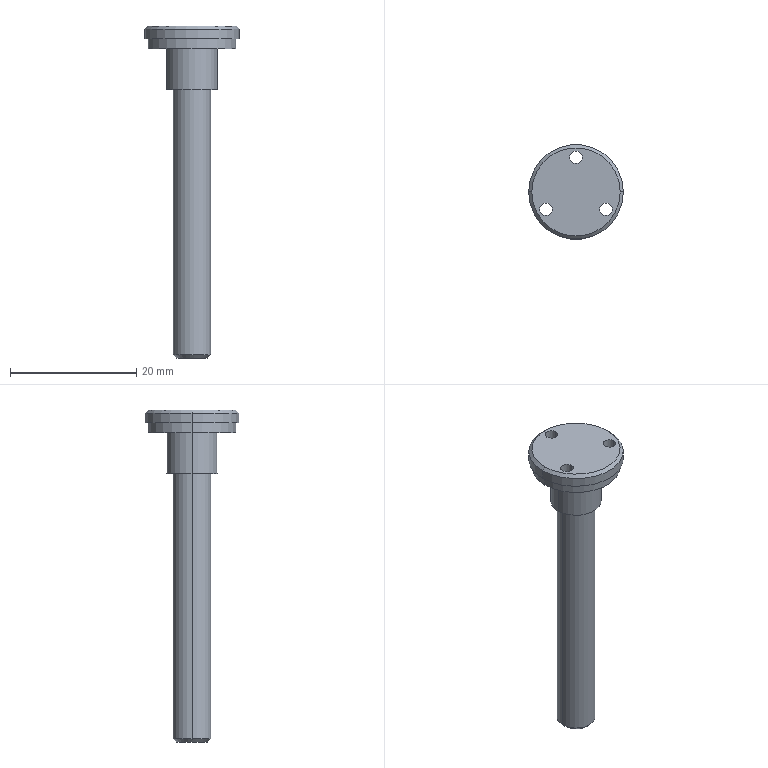Part | NX | features BREP 1 | 1 solid | 26 faces | box 15 x 15 x 52.6 mm | volume 2030 mm3 | cylinder 16 | plane 6 | cone 4 | commonest cylinder face diameters 2 x6 3.1 x2 6 x2 8 x2 13.9 x2 15 x2
STEP:
#1=CARTESIAN_POINT('',(-165.024,187.29,-49.6));
#2=VERTEX_POINT('',#1);
#3=CARTESIAN_POINT('',(-160.024,187.29,-49.6));
#4=VERTEX_POINT('',#3);
#5=CARTESIAN_POINT('',(-162.524,187.29,-49.6));
#6=DIRECTION('',(0.,0.,-1.));
#7=DIRECTION('',(1.,0.,0.));
#8=AXIS2_PLACEMENT_3D('',#5,#6,#7);
#9=CIRCLE('',#8,2.5);
#10=EDGE_CURVE('',#2,#4,#9,.T.);
#11=ORIENTED_EDGE('',*,*,#10,.F.);
#12=CARTESIAN_POINT('',(-165.524,187.29,-49.1));
#13=VERTEX_POINT('',#12);
#14=CARTESIAN_POINT('',(-165.024,187.29,-49.6));
#15=DIRECTION('',(-0.7071,0.,0.7071));
#16=VECTOR('',#15,1000.);
#17=LINE('',#14,#16);
#18=EDGE_CURVE('',#2,#13,#17,.T.);
#19=ORIENTED_EDGE('',*,*,#18,.T.);
#20=CARTESIAN_POINT('',(-159.524,187.29,-49.1));
#21=VERTEX_POINT('',#20);
#22=CARTESIAN_POINT('',(-162.524,187.29,-49.1));
#23=DIRECTION('',(0.,0.,1.));
#24=DIRECTION('',(1.,0.,0.));
#25=AXIS2_PLACEMENT_3D('',#22,#23,#24);
#26=CIRCLE('',#25,3.);
#27=EDGE_CURVE('',#21,#13,#26,.T.);
#28=ORIENTED_EDGE('',*,*,#27,.F.);
#29=CARTESIAN_POINT('',(-160.024,187.29,-49.6));
#30=DIRECTION('',(0.7071,0.,0.7071));
#31=VECTOR('',#30,1000.);
#32=LINE('',#29,#31);
#33=EDGE_CURVE('',#4,#21,#32,.T.);
#34=ORIENTED_EDGE('',*,*,#33,.F.);
#35=EDGE_LOOP('',(#11,#19,#28,#34));
#36=FACE_BOUND('',#35,.T.);
#37=CARTESIAN_POINT('',(-162.524,187.29,-49.6));
#38=DIRECTION('',(0.,0.,1.));
#39=DIRECTION('',(-1.,0.,0.));
#40=AXIS2_PLACEMENT_3D('',#37,#38,#39);
#41=CONICAL_SURFACE('',#40,2.5,0.7854);
#42=ADVANCED_FACE('',(#36),#41,.T.);
#43=CARTESIAN_POINT('',(-155.524,187.29,3.));
#44=VERTEX_POINT('',#43);
#45=CARTESIAN_POINT('',(-169.524,187.29,3.));
#46=VERTEX_POINT('',#45);
#47=CARTESIAN_POINT('',(-162.524,187.29,3.));
#48=DIRECTION('',(0.,0.,1.));
#49=DIRECTION('',(1.,0.,0.));
#50=AXIS2_PLACEMENT_3D('',#47,#48,#49);
#51=CIRCLE('',#50,7.);
#52=EDGE_CURVE('',#44,#46,#51,.T.);
#53=ORIENTED_EDGE('',*,*,#52,.F.);
#54=CARTESIAN_POINT('',(-155.024,187.29,2.5));
#55=VERTEX_POINT('',#54);
#56=CARTESIAN_POINT('',(-155.524,187.29,3.));
#57=DIRECTION('',(0.7071,0.,-0.7071));
#58=VECTOR('',#57,1000.);
#59=LINE('',#56,#58);
#60=EDGE_CURVE('',#55,#44,#59,.F.);
#61=ORIENTED_EDGE('',*,*,#60,.F.);
#62=CARTESIAN_POINT('',(-170.024,187.29,2.5));
#63=VERTEX_POINT('',#62);
#64=CARTESIAN_POINT('',(-162.524,187.29,2.5));
#65=DIRECTION('',(0.,0.,-1.));
#66=DIRECTION('',(1.,0.,0.));
#67=AXIS2_PLACEMENT_3D('',#64,#65,#66);
#68=CIRCLE('',#67,7.5);
#69=EDGE_CURVE('',#63,#55,#68,.T.);
#70=ORIENTED_EDGE('',*,*,#69,.F.);
#71=CARTESIAN_POINT('',(-169.524,187.29,3.));
#72=DIRECTION('',(-0.7071,0.,-0.7071));
#73=VECTOR('',#72,1000.);
#74=LINE('',#71,#73);
#75=EDGE_CURVE('',#63,#46,#74,.F.);
#76=ORIENTED_EDGE('',*,*,#75,.T.);
#77=EDGE_LOOP('',(#53,#61,#70,#76));
#78=FACE_BOUND('',#77,.T.);
#79=CARTESIAN_POINT('',(-162.524,187.29,3.));
#80=DIRECTION('',(0.,0.,-1.));
#81=DIRECTION('',(1.,0.,0.));
#82=AXIS2_PLACEMENT_3D('',#79,#80,#81);
#83=CONICAL_SURFACE('',#82,7.,0.7854);
#84=ADVANCED_FACE('',(#78),#83,.T.);
#85=CARTESIAN_POINT('',(-163.524,192.79,3.));
#86=VERTEX_POINT('',#85);
#87=CARTESIAN_POINT('',(-161.524,192.79,3.));
#88=VERTEX_POINT('',#87);
#89=CARTESIAN_POINT('',(-162.524,192.79,3.));
#90=DIRECTION('',(0.,0.,1.));
#91=DIRECTION('',(1.,0.,0.));
#92=AXIS2_PLACEMENT_3D('',#89,#90,#91);
#93=CIRCLE('',#92,1.);
#94=EDGE_CURVE('',#86,#88,#93,.T.);
#95=ORIENTED_EDGE('',*,*,#94,.T.);
#96=CARTESIAN_POINT('',(-161.524,192.79,-0.6));
#97=VERTEX_POINT('',#96);
#98=CARTESIAN_POINT('',(-161.524,192.79,9.4));
#99=DIRECTION('',(0.,0.,-1.));
#100=VECTOR('',#99,1000.);
#101=LINE('',#98,#100);
#102=EDGE_CURVE('',#97,#88,#101,.F.);
#103=ORIENTED_EDGE('',*,*,#102,.F.);
#104=CARTESIAN_POINT('',(-163.524,192.79,-0.6));
#105=VERTEX_POINT('',#104);
#106=CARTESIAN_POINT('',(-162.524,192.79,-0.6));
#107=DIRECTION('',(0.,0.,-1.));
#108=DIRECTION('',(-1.,0.,0.));
#109=AXIS2_PLACEMENT_3D('',#106,#107,#108);
#110=CIRCLE('',#109,1.);
#111=EDGE_CURVE('',#97,#105,#110,.T.);
#112=ORIENTED_EDGE('',*,*,#111,.T.);
#113=CARTESIAN_POINT('',(-163.524,192.79,9.4));
#114=DIRECTION('',(0.,0.,-1.));
#115=VECTOR('',#114,1000.);
#116=LINE('',#113,#115);
#117=EDGE_CURVE('',#105,#86,#116,.F.);
#118=ORIENTED_EDGE('',*,*,#117,.T.);
#119=EDGE_LOOP('',(#95,#103,#112,#118));
#120=FACE_BOUND('',#119,.T.);
#121=CARTESIAN_POINT('',(-162.524,192.79,9.4));
#122=DIRECTION('',(0.,0.,-1.));
#123=DIRECTION('',(1.,0.,0.));
#124=AXIS2_PLACEMENT_3D('',#121,#122,#123);
#125=CYLINDRICAL_SURFACE('',#124,1.);
#126=ADVANCED_FACE('',(#120),#125,.F.);
#127=CARTESIAN_POINT('',(-168.288,184.54,3.));
#128=VERTEX_POINT('',#127);
#129=CARTESIAN_POINT('',(-166.288,184.54,3.));
#130=VERTEX_POINT('',#129);
#131=CARTESIAN_POINT('',(-167.288,184.54,3.));
#132=DIRECTION('',(0.,0.,1.));
#133=DIRECTION('',(1.,0.,0.));
#134=AXIS2_PLACEMENT_3D('',#131,#132,#133);
#135=CIRCLE('',#134,1.);
#136=EDGE_CURVE('',#128,#130,#135,.T.);
#137=ORIENTED_EDGE('',*,*,#136,.T.);
#138=CARTESIAN_POINT('',(-166.288,184.54,-0.6));
#139=VERTEX_POINT('',#138);
#140=CARTESIAN_POINT('',(-166.288,184.54,9.4));
#141=DIRECTION('',(0.,0.,-1.));
#142=VECTOR('',#141,1000.);
#143=LINE('',#140,#142);
#144=EDGE_CURVE('',#139,#130,#143,.F.);
#145=ORIENTED_EDGE('',*,*,#144,.F.);
#146=CARTESIAN_POINT('',(-168.288,184.54,-0.6));
#147=VERTEX_POINT('',#146);
#148=CARTESIAN_POINT('',(-167.288,184.54,-0.6));
#149=DIRECTION('',(0.,0.,-1.));
#150=DIRECTION('',(-1.,0.,0.));
#151=AXIS2_PLACEMENT_3D('',#148,#149,#150);
#152=CIRCLE('',#151,1.);
#153=EDGE_CURVE('',#139,#147,#152,.T.);
#154=ORIENTED_EDGE('',*,*,#153,.T.);
#155=CARTESIAN_POINT('',(-168.288,184.54,9.4));
#156=DIRECTION('',(0.,0.,-1.));
#157=VECTOR('',#156,1000.);
#158=LINE('',#155,#157);
#159=EDGE_CURVE('',#147,#128,#158,.F.);
#160=ORIENTED_EDGE('',*,*,#159,.T.);
#161=EDGE_LOOP('',(#137,#145,#154,#160));
#162=FACE_BOUND('',#161,.T.);
#163=CARTESIAN_POINT('',(-167.288,184.54,9.4));
#164=DIRECTION('',(0.,0.,-1.));
#165=DIRECTION('',(1.,0.,0.));
#166=AXIS2_PLACEMENT_3D('',#163,#164,#165);
#167=CYLINDRICAL_SURFACE('',#166,1.);
#168=ADVANCED_FACE('',(#162),#167,.F.);
#169=CARTESIAN_POINT('',(-158.761,184.54,3.));
#170=VERTEX_POINT('',#169);
#171=CARTESIAN_POINT('',(-156.761,184.54,3.));
#172=VERTEX_POINT('',#171);
#173=CARTESIAN_POINT('',(-157.761,184.54,3.));
#174=DIRECTION('',(0.,0.,1.));
#175=DIRECTION('',(1.,0.,0.));
#176=AXIS2_PLACEMENT_3D('',#173,#174,#175);
#177=CIRCLE('',#176,1.);
#178=EDGE_CURVE('',#170,#172,#177,.T.);
#179=ORIENTED_EDGE('',*,*,#178,.T.);
#180=CARTESIAN_POINT('',(-156.761,184.54,-0.6));
#181=VERTEX_POINT('',#180);
#182=CARTESIAN_POINT('',(-156.761,184.54,9.4));
#183=DIRECTION('',(0.,0.,-1.));
#184=VECTOR('',#183,1000.);
#185=LINE('',#182,#184);
#186=EDGE_CURVE('',#181,#172,#185,.F.);
#187=ORIENTED_EDGE('',*,*,#186,.F.);
#188=CARTESIAN_POINT('',(-158.761,184.54,-0.6));
#189=VERTEX_POINT('',#188);
#190=CARTESIAN_POINT('',(-157.761,184.54,-0.6));
#191=DIRECTION('',(0.,0.,-1.));
#192=DIRECTION('',(-1.,0.,0.));
#193=AXIS2_PLACEMENT_3D('',#190,#191,#192);
#194=CIRCLE('',#193,1.);
#195=EDGE_CURVE('',#181,#189,#194,.T.);
#196=ORIENTED_EDGE('',*,*,#195,.T.);
#197=CARTESIAN_POINT('',(-158.761,184.54,9.4));
#198=DIRECTION('',(0.,0.,-1.));
#199=VECTOR('',#198,1000.);
#200=LINE('',#197,#199);
#201=EDGE_CURVE('',#189,#170,#200,.F.);
#202=ORIENTED_EDGE('',*,*,#201,.T.);
#203=EDGE_LOOP('',(#179,#187,#196,#202));
#204=FACE_BOUND('',#203,.T.);
#205=CARTESIAN_POINT('',(-157.761,184.54,9.4));
#206=DIRECTION('',(0.,0.,-1.));
#207=DIRECTION('',(1.,0.,0.));
#208=AXIS2_PLACEMENT_3D('',#205,#206,#207);
#209=CYLINDRICAL_SURFACE('',#208,1.);
#210=ADVANCED_FACE('',(#204),#209,.F.);
#211=ORIENTED_EDGE('',*,*,#69,.T.);
#212=CARTESIAN_POINT('',(-155.024,187.29,1.));
#213=VERTEX_POINT('',#212);
#214=CARTESIAN_POINT('',(-155.024,187.29,2.));
#215=DIRECTION('',(0.,0.,-1.));
#216=VECTOR('',#215,1000.);
#217=LINE('',#214,#216);
#218=EDGE_CURVE('',#213,#55,#217,.F.);
#219=ORIENTED_EDGE('',*,*,#218,.F.);
#220=CARTESIAN_POINT('',(-170.024,187.29,1.));
#221=VERTEX_POINT('',#220);
#222=CARTESIAN_POINT('',(-162.524,187.29,1.));
#223=DIRECTION('',(0.,0.,1.));
#224=DIRECTION('',(1.,0.,0.));
#225=AXIS2_PLACEMENT_3D('',#222,#223,#224);
#226=CIRCLE('',#225,7.5);
#227=EDGE_CURVE('',#213,#221,#226,.T.);
#228=ORIENTED_EDGE('',*,*,#227,.T.);
#229=CARTESIAN_POINT('',(-170.024,187.29,2.));
#230=DIRECTION('',(0.,0.,-1.));
#231=VECTOR('',#230,1000.);
#232=LINE('',#229,#231);
#233=EDGE_CURVE('',#221,#63,#232,.F.);
#234=ORIENTED_EDGE('',*,*,#233,.T.);
#235=EDGE_LOOP('',(#211,#219,#228,#234));
#236=FACE_BOUND('',#235,.T.);
#237=CARTESIAN_POINT('',(-162.524,187.29,2.));
#238=DIRECTION('',(0.,0.,-1.));
#239=DIRECTION('',(1.,0.,0.));
#240=AXIS2_PLACEMENT_3D('',#237,#238,#239);
#241=CYLINDRICAL_SURFACE('',#240,7.5);
#242=ADVANCED_FACE('',(#236),#241,.T.);
#243=CARTESIAN_POINT('',(-169.474,187.29,-0.6));
#244=VERTEX_POINT('',#243);
#245=CARTESIAN_POINT('',(-155.574,187.29,-0.6));
#246=VERTEX_POINT('',#245);
#247=CARTESIAN_POINT('',(-162.524,187.29,-0.6));
#248=DIRECTION('',(0.,0.,-1.));
#249=DIRECTION('',(-1.,0.,0.));
#250=AXIS2_PLACEMENT_3D('',#247,#248,#249);
#251=CIRCLE('',#250,6.95);
#252=EDGE_CURVE('',#244,#246,#251,.T.);
#253=ORIENTED_EDGE('',*,*,#252,.F.);
#254=CARTESIAN_POINT('',(-169.474,187.29,1.));
#255=VERTEX_POINT('',#254);
#256=CARTESIAN_POINT('',(-169.474,187.29,-20.258));
#257=DIRECTION('',(0.,0.,1.));
#258=VECTOR('',#257,1000.);
#259=LINE('',#256,#258);
#260=EDGE_CURVE('',#244,#255,#259,.T.);
#261=ORIENTED_EDGE('',*,*,#260,.T.);
#262=CARTESIAN_POINT('',(-155.574,187.29,1.));
#263=VERTEX_POINT('',#262);
#264=CARTESIAN_POINT('',(-162.524,187.29,1.));
#265=DIRECTION('',(0.,0.,-1.));
#266=DIRECTION('',(1.,0.,0.));
#267=AXIS2_PLACEMENT_3D('',#264,#265,#266);
#268=CIRCLE('',#267,6.95);
#269=EDGE_CURVE('',#255,#263,#268,.T.);
#270=ORIENTED_EDGE('',*,*,#269,.T.);
#271=CARTESIAN_POINT('',(-155.574,187.29,-20.258));
#272=DIRECTION('',(0.,0.,1.));
#273=VECTOR('',#272,1000.);
#274=LINE('',#271,#273);
#275=EDGE_CURVE('',#246,#263,#274,.T.);
#276=ORIENTED_EDGE('',*,*,#275,.F.);
#277=EDGE_LOOP('',(#253,#261,#270,#276));
#278=FACE_BOUND('',#277,.T.);
#279=CARTESIAN_POINT('',(-162.524,187.29,-20.258));
#280=DIRECTION('',(0.,0.,1.));
#281=DIRECTION('',(-1.,0.,0.));
#282=AXIS2_PLACEMENT_3D('',#279,#280,#281);
#283=CYLINDRICAL_SURFACE('',#282,6.95);
#284=ADVANCED_FACE('',(#278),#283,.T.);
#285=CARTESIAN_POINT('',(-166.524,187.29,-7.1));
#286=VERTEX_POINT('',#285);
#287=CARTESIAN_POINT('',(-158.524,187.29,-7.1));
#288=VERTEX_POINT('',#287);
#289=CARTESIAN_POINT('',(-162.524,187.29,-7.1));
#290=DIRECTION('',(0.,0.,-1.));
#291=DIRECTION('',(-1.,0.,0.));
#292=AXIS2_PLACEMENT_3D('',#289,#290,#291);
#293=CIRCLE('',#292,4.);
#294=EDGE_CURVE('',#286,#288,#293,.T.);
#295=ORIENTED_EDGE('',*,*,#294,.F.);
#296=CARTESIAN_POINT('',(-166.524,187.29,-0.6));
#297=VERTEX_POINT('',#296);
#298=CARTESIAN_POINT('',(-166.524,187.29,-18.514));
#299=DIRECTION('',(0.,0.,1.));
#300=VECTOR('',#299,1000.);
#301=LINE('',#298,#300);
#302=EDGE_CURVE('',#286,#297,#301,.T.);
#303=ORIENTED_EDGE('',*,*,#302,.T.);
#304=CARTESIAN_POINT('',(-158.524,187.29,-0.6));
#305=VERTEX_POINT('',#304);
#306=CARTESIAN_POINT('',(-162.524,187.29,-0.6));
#307=DIRECTION('',(0.,0.,-1.));
#308=DIRECTION('',(-1.,0.,0.));
#309=AXIS2_PLACEMENT_3D('',#306,#307,#308);
#310=CIRCLE('',#309,4.);
#311=EDGE_CURVE('',#297,#305,#310,.T.);
#312=ORIENTED_EDGE('',*,*,#311,.T.);
#313=CARTESIAN_POINT('',(-158.524,187.29,-18.514));
#314=DIRECTION('',(0.,0.,1.));
#315=VECTOR('',#314,1000.);
#316=LINE('',#313,#315);
#317=EDGE_CURVE('',#288,#305,#316,.T.);
#318=ORIENTED_EDGE('',*,*,#317,.F.);
#319=EDGE_LOOP('',(#295,#303,#312,#318));
#320=FACE_BOUND('',#319,.T.);
#321=CARTESIAN_POINT('',(-162.524,187.29,-18.514));
#322=DIRECTION('',(0.,0.,1.));
#323=DIRECTION('',(-1.,0.,0.));
#324=AXIS2_PLACEMENT_3D('',#321,#322,#323);
#325=CYLINDRICAL_SURFACE('',#324,4.);
#326=ADVANCED_FACE('',(#320),#325,.T.);
#327=CARTESIAN_POINT('',(-160.974,187.29,-42.6));
#328=VERTEX_POINT('',#327);
#329=CARTESIAN_POINT('',(-164.074,187.29,-42.6));
#330=VERTEX_POINT('',#329);
#331=CARTESIAN_POINT('',(-162.524,187.29,-42.6));
#332=DIRECTION('',(0.,0.,-1.));
#333=DIRECTION('',(-1.,0.,0.));
#334=AXIS2_PLACEMENT_3D('',#331,#332,#333);
#335=CIRCLE('',#334,1.55);
#336=EDGE_CURVE('',#328,#330,#335,.T.);
#337=ORIENTED_EDGE('',*,*,#336,.F.);
#338=CARTESIAN_POINT('',(-160.974,187.29,-49.6));
#339=VERTEX_POINT('',#338);
#340=CARTESIAN_POINT('',(-160.974,187.29,-42.6));
#341=DIRECTION('',(0.,0.,-1.));
#342=VECTOR('',#341,1000.);
#343=LINE('',#340,#342);
#344=EDGE_CURVE('',#339,#328,#343,.F.);
#345=ORIENTED_EDGE('',*,*,#344,.F.);
#346=CARTESIAN_POINT('',(-164.074,187.29,-49.6));
#347=VERTEX_POINT('',#346);
#348=CARTESIAN_POINT('',(-162.524,187.29,-49.6));
#349=DIRECTION('',(0.,0.,-1.));
#350=DIRECTION('',(1.,0.,0.));
#351=AXIS2_PLACEMENT_3D('',#348,#349,#350);
#352=CIRCLE('',#351,1.55);
#353=EDGE_CURVE('',#339,#347,#352,.T.);
#354=ORIENTED_EDGE('',*,*,#353,.T.);
#355=CARTESIAN_POINT('',(-164.074,187.29,-42.6));
#356=DIRECTION('',(0.,0.,-1.));
#357=VECTOR('',#356,1000.);
#358=LINE('',#355,#357);
#359=EDGE_CURVE('',#347,#330,#358,.F.);
#360=ORIENTED_EDGE('',*,*,#359,.T.);
#361=EDGE_LOOP('',(#337,#345,#354,#360));
#362=FACE_BOUND('',#361,.T.);
#363=CARTESIAN_POINT('',(-162.524,187.29,-42.6));
#364=DIRECTION('',(0.,0.,-1.));
#365=DIRECTION('',(1.,0.,0.));
#366=AXIS2_PLACEMENT_3D('',#363,#364,#365);
#367=CYLINDRICAL_SURFACE('',#366,1.55);
#368=ADVANCED_FACE('',(#362),#367,.F.);
#369=ORIENTED_EDGE('',*,*,#27,.T.);
#370=CARTESIAN_POINT('',(-165.524,187.29,-7.1));
#371=VERTEX_POINT('',#370);
#372=CARTESIAN_POINT('',(-165.524,187.29,-61.085));
#373=DIRECTION('',(0.,0.,1.));
#374=VECTOR('',#373,1000.);
#375=LINE('',#372,#374);
#376=EDGE_CURVE('',#13,#371,#375,.T.);
#377=ORIENTED_EDGE('',*,*,#376,.T.);
#378=CARTESIAN_POINT('',(-159.524,187.29,-7.1));
#379=VERTEX_POINT('',#378);
#380=CARTESIAN_POINT('',(-162.524,187.29,-7.1));
#381=DIRECTION('',(0.,0.,1.));
#382=DIRECTION('',(-1.,0.,0.));
#383=AXIS2_PLACEMENT_3D('',#380,#381,#382);
#384=CIRCLE('',#383,3.);
#385=EDGE_CURVE('',#379,#371,#384,.T.);
#386=ORIENTED_EDGE('',*,*,#385,.F.);
#387=CARTESIAN_POINT('',(-159.524,187.29,-61.085));
#388=DIRECTION('',(0.,0.,1.));
#389=VECTOR('',#388,1000.);
#390=LINE('',#387,#389);
#391=EDGE_CURVE('',#21,#379,#390,.T.);
#392=ORIENTED_EDGE('',*,*,#391,.F.);
#393=EDGE_LOOP('',(#369,#377,#386,#392));
#394=FACE_BOUND('',#393,.T.);
#395=CARTESIAN_POINT('',(-162.524,187.29,-61.085));
#396=DIRECTION('',(0.,0.,1.));
#397=DIRECTION('',(-1.,0.,0.));
#398=AXIS2_PLACEMENT_3D('',#395,#396,#397);
#399=CYLINDRICAL_SURFACE('',#398,3.);
#400=ADVANCED_FACE('',(#394),#399,.T.);
#401=ORIENTED_EDGE('',*,*,#376,.F.);
#402=CARTESIAN_POINT('',(-162.524,187.29,-49.1));
#403=DIRECTION('',(0.,0.,1.));
#404=DIRECTION('',(1.,0.,0.));
#405=AXIS2_PLACEMENT_3D('',#402,#403,#404);
#406=CIRCLE('',#405,3.);
#407=EDGE_CURVE('',#13,#21,#406,.T.);
#408=ORIENTED_EDGE('',*,*,#407,.T.);
#409=ORIENTED_EDGE('',*,*,#391,.T.);
#410=CARTESIAN_POINT('',(-162.524,187.29,-7.1));
#411=DIRECTION('',(0.,0.,1.));
#412=DIRECTION('',(-1.,0.,0.));
#413=AXIS2_PLACEMENT_3D('',#410,#411,#412);
#414=CIRCLE('',#413,3.);
#415=EDGE_CURVE('',#371,#379,#414,.T.);
#416=ORIENTED_EDGE('',*,*,#415,.F.);
#417=EDGE_LOOP('',(#401,#408,#409,#416));
#418=FACE_BOUND('',#417,.T.);
#419=CARTESIAN_POINT('',(-162.524,187.29,-61.085));
#420=DIRECTION('',(0.,0.,1.));
#421=DIRECTION('',(-1.,0.,0.));
#422=AXIS2_PLACEMENT_3D('',#419,#420,#421);
#423=CYLINDRICAL_SURFACE('',#422,3.);
#424=ADVANCED_FACE('',(#418),#423,.T.);
#425=CARTESIAN_POINT('',(-162.524,187.29,-49.6));
#426=DIRECTION('',(0.,0.,-1.));
#427=DIRECTION('',(1.,0.,0.));
#428=AXIS2_PLACEMENT_3D('',#425,#426,#427);
#429=CIRCLE('',#428,2.5);
#430=EDGE_CURVE('',#4,#2,#429,.T.);
#431=ORIENTED_EDGE('',*,*,#430,.T.);
#432=ORIENTED_EDGE('',*,*,#10,.T.);
#433=EDGE_LOOP('',(#431,#432));
#434=FACE_BOUND('',#433,.T.);
#435=CARTESIAN_POINT('',(-162.524,187.29,-49.6));
#436=DIRECTION('',(0.,0.,-1.));
#437=DIRECTION('',(1.,0.,0.));
#438=AXIS2_PLACEMENT_3D('',#435,#436,#437);
#439=CIRCLE('',#438,1.55);
#440=EDGE_CURVE('',#347,#339,#439,.T.);
#441=ORIENTED_EDGE('',*,*,#440,.F.);
#442=ORIENTED_EDGE('',*,*,#353,.F.);
#443=EDGE_LOOP('',(#441,#442));
#444=FACE_BOUND('',#443,.T.);
#445=CARTESIAN_POINT('',(-156.998,188.192,-49.6));
#446=DIRECTION('',(0.,0.,1.));
#447=DIRECTION('',(-1.,0.,0.));
#448=AXIS2_PLACEMENT_3D('',#445,#446,#447);
#449=PLANE('',#448);
#450=ADVANCED_FACE('',(#434,#444),#449,.F.);
#451=ORIENTED_EDGE('',*,*,#344,.T.);
#452=CARTESIAN_POINT('',(-162.524,187.29,-42.6));
#453=DIRECTION('',(0.,0.,-1.));
#454=DIRECTION('',(-1.,0.,0.));
#455=AXIS2_PLACEMENT_3D('',#452,#453,#454);
#456=CIRCLE('',#455,1.55);
#457=EDGE_CURVE('',#330,#328,#456,.T.);
#458=ORIENTED_EDGE('',*,*,#457,.F.);
#459=ORIENTED_EDGE('',*,*,#359,.F.);
#460=ORIENTED_EDGE('',*,*,#440,.T.);
#461=EDGE_LOOP('',(#451,#458,#459,#460));
#462=FACE_BOUND('',#461,.T.);
#463=CARTESIAN_POINT('',(-162.524,187.29,-42.6));
#464=DIRECTION('',(0.,0.,-1.));
#465=DIRECTION('',(1.,0.,0.));
#466=AXIS2_PLACEMENT_3D('',#463,#464,#465);
#467=CYLINDRICAL_SURFACE('',#466,1.55);
#468=ADVANCED_FACE('',(#462),#467,.F.);
#469=ORIENTED_EDGE('',*,*,#457,.T.);
#470=ORIENTED_EDGE('',*,*,#336,.T.);
#471=EDGE_LOOP('',(#469,#470));
#472=FACE_BOUND('',#471,.T.);
#473=CARTESIAN_POINT('',(-162.524,187.29,-42.6));
#474=DIRECTION('',(0.,0.,-1.));
#475=DIRECTION('',(0.,1.,0.));
#476=AXIS2_PLACEMENT_3D('',#473,#474,#475);
#477=PLANE('',#476);
#478=ADVANCED_FACE('',(#472),#477,.T.);
#479=ORIENTED_EDGE('',*,*,#302,.F.);
#480=CARTESIAN_POINT('',(-162.524,187.29,-7.1));
#481=DIRECTION('',(0.,0.,-1.));
#482=DIRECTION('',(-1.,0.,0.));
#483=AXIS2_PLACEMENT_3D('',#480,#481,#482);
#484=CIRCLE('',#483,4.);
#485=EDGE_CURVE('',#288,#286,#484,.T.);
#486=ORIENTED_EDGE('',*,*,#485,.F.);
#487=ORIENTED_EDGE('',*,*,#317,.T.);
#488=CARTESIAN_POINT('',(-162.524,187.29,-0.6));
#489=DIRECTION('',(0.,0.,-1.));
#490=DIRECTION('',(-1.,0.,0.));
#491=AXIS2_PLACEMENT_3D('',#488,#489,#490);
#492=CIRCLE('',#491,4.);
#493=EDGE_CURVE('',#305,#297,#492,.T.);
#494=ORIENTED_EDGE('',*,*,#493,.T.);
#495=EDGE_LOOP('',(#479,#486,#487,#494));
#496=FACE_BOUND('',#495,.T.);
#497=CARTESIAN_POINT('',(-162.524,187.29,-18.514));
#498=DIRECTION('',(0.,0.,1.));
#499=DIRECTION('',(-1.,0.,0.));
#500=AXIS2_PLACEMENT_3D('',#497,#498,#499);
#501=CYLINDRICAL_SURFACE('',#500,4.);
#502=ADVANCED_FACE('',(#496),#501,.T.);
#503=ORIENTED_EDGE('',*,*,#485,.T.);
#504=ORIENTED_EDGE('',*,*,#294,.T.);
#505=EDGE_LOOP('',(#503,#504));
#506=FACE_BOUND('',#505,.T.);
#507=ORIENTED_EDGE('',*,*,#385,.T.);
#508=ORIENTED_EDGE('',*,*,#415,.T.);
#509=EDGE_LOOP('',(#507,#508));
#510=FACE_BOUND('',#509,.T.);
#511=CARTESIAN_POINT('',(-164.736,192.434,-7.1));
#512=DIRECTION('',(0.,0.,-1.));
#513=DIRECTION('',(0.,1.,0.));
#514=AXIS2_PLACEMENT_3D('',#511,#512,#513);
#515=PLANE('',#514);
#516=ADVANCED_FACE('',(#506,#510),#515,.T.);
#517=ORIENTED_EDGE('',*,*,#260,.F.);
#518=CARTESIAN_POINT('',(-162.524,187.29,-0.6));
#519=DIRECTION('',(0.,0.,-1.));
#520=DIRECTION('',(-1.,0.,0.));
#521=AXIS2_PLACEMENT_3D('',#518,#519,#520);
#522=CIRCLE('',#521,6.95);
#523=EDGE_CURVE('',#246,#244,#522,.T.);
#524=ORIENTED_EDGE('',*,*,#523,.F.);
#525=ORIENTED_EDGE('',*,*,#275,.T.);
#526=CARTESIAN_POINT('',(-162.524,187.29,1.));
#527=DIRECTION('',(0.,0.,-1.));
#528=DIRECTION('',(1.,0.,0.));
#529=AXIS2_PLACEMENT_3D('',#526,#527,#528);
#530=CIRCLE('',#529,6.95);
#531=EDGE_CURVE('',#263,#255,#530,.T.);
#532=ORIENTED_EDGE('',*,*,#531,.T.);
#533=EDGE_LOOP('',(#517,#524,#525,#532));
#534=FACE_BOUND('',#533,.T.);
#535=CARTESIAN_POINT('',(-162.524,187.29,-20.258));
#536=DIRECTION('',(0.,0.,1.));
#537=DIRECTION('',(-1.,0.,0.));
#538=AXIS2_PLACEMENT_3D('',#535,#536,#537);
#539=CYLINDRICAL_SURFACE('',#538,6.95);
#540=ADVANCED_FACE('',(#534),#539,.T.);
#541=ORIENTED_EDGE('',*,*,#523,.T.);
#542=ORIENTED_EDGE('',*,*,#252,.T.);
#543=EDGE_LOOP('',(#541,#542));
#544=FACE_BOUND('',#543,.T.);
#545=CARTESIAN_POINT('',(-162.524,192.79,-0.6));
#546=DIRECTION('',(0.,0.,-1.));
#547=DIRECTION('',(-1.,0.,0.));
#548=AXIS2_PLACEMENT_3D('',#545,#546,#547);
#549=CIRCLE('',#548,1.);
#550=EDGE_CURVE('',#105,#97,#549,.T.);
#551=ORIENTED_EDGE('',*,*,#550,.F.);
#552=ORIENTED_EDGE('',*,*,#111,.F.);
#553=EDGE_LOOP('',(#551,#552));
#554=FACE_BOUND('',#553,.T.);
#555=CARTESIAN_POINT('',(-167.288,184.54,-0.6));
#556=DIRECTION('',(0.,0.,-1.));
#557=DIRECTION('',(-1.,0.,0.));
#558=AXIS2_PLACEMENT_3D('',#555,#556,#557);
#559=CIRCLE('',#558,1.);
#560=EDGE_CURVE('',#147,#139,#559,.T.);
#561=ORIENTED_EDGE('',*,*,#560,.F.);
#562=ORIENTED_EDGE('',*,*,#153,.F.);
#563=EDGE_LOOP('',(#561,#562));
#564=FACE_BOUND('',#563,.T.);
#565=CARTESIAN_POINT('',(-157.761,184.54,-0.6));
#566=DIRECTION('',(0.,0.,-1.));
#567=DIRECTION('',(-1.,0.,0.));
#568=AXIS2_PLACEMENT_3D('',#565,#566,#567);
#569=CIRCLE('',#568,1.);
#570=EDGE_CURVE('',#189,#181,#569,.T.);
#571=ORIENTED_EDGE('',*,*,#570,.F.);
#572=ORIENTED_EDGE('',*,*,#195,.F.);
#573=EDGE_LOOP('',(#571,#572));
#574=FACE_BOUND('',#573,.T.);
#575=ORIENTED_EDGE('',*,*,#493,.F.);
#576=ORIENTED_EDGE('',*,*,#311,.F.);
#577=EDGE_LOOP('',(#575,#576));
#578=FACE_BOUND('',#577,.T.);
#579=CARTESIAN_POINT('',(-171.196,182.31,-0.6));
#580=DIRECTION('',(0.,0.,-1.));
#581=DIRECTION('',(1.,0.,0.));
#582=AXIS2_PLACEMENT_3D('',#579,#580,#581);
#583=PLANE('',#582);
#584=ADVANCED_FACE('',(#544,#554,#564,#574,#578),#583,.T.);
#585=CARTESIAN_POINT('',(-162.524,187.29,3.));
#586=DIRECTION('',(0.,0.,1.));
#587=DIRECTION('',(1.,0.,0.));
#588=AXIS2_PLACEMENT_3D('',#585,#586,#587);
#589=CIRCLE('',#588,7.);
#590=EDGE_CURVE('',#46,#44,#589,.T.);
#591=ORIENTED_EDGE('',*,*,#590,.T.);
#592=ORIENTED_EDGE('',*,*,#52,.T.);
#593=EDGE_LOOP('',(#591,#592));
#594=FACE_BOUND('',#593,.T.);
#595=ORIENTED_EDGE('',*,*,#94,.F.);
#596=CARTESIAN_POINT('',(-162.524,192.79,3.));
#597=DIRECTION('',(0.,0.,1.));
#598=DIRECTION('',(1.,0.,0.));
#599=AXIS2_PLACEMENT_3D('',#596,#597,#598);
#600=CIRCLE('',#599,1.);
#601=EDGE_CURVE('',#88,#86,#600,.T.);
#602=ORIENTED_EDGE('',*,*,#601,.F.);
#603=EDGE_LOOP('',(#595,#602));
#604=FACE_BOUND('',#603,.T.);
#605=ORIENTED_EDGE('',*,*,#136,.F.);
#606=CARTESIAN_POINT('',(-167.288,184.54,3.));
#607=DIRECTION('',(0.,0.,1.));
#608=DIRECTION('',(1.,0.,0.));
#609=AXIS2_PLACEMENT_3D('',#606,#607,#608);
#610=CIRCLE('',#609,1.);
#611=EDGE_CURVE('',#130,#128,#610,.T.);
#612=ORIENTED_EDGE('',*,*,#611,.F.);
#613=EDGE_LOOP('',(#605,#612));
#614=FACE_BOUND('',#613,.T.);
#615=ORIENTED_EDGE('',*,*,#178,.F.);
#616=CARTESIAN_POINT('',(-157.761,184.54,3.));
#617=DIRECTION('',(0.,0.,1.));
#618=DIRECTION('',(1.,0.,0.));
#619=AXIS2_PLACEMENT_3D('',#616,#617,#618);
#620=CIRCLE('',#619,1.);
#621=EDGE_CURVE('',#172,#170,#620,.T.);
#622=ORIENTED_EDGE('',*,*,#621,.F.);
#623=EDGE_LOOP('',(#615,#622));
#624=FACE_BOUND('',#623,.T.);
#625=CARTESIAN_POINT('',(-162.524,187.29,3.));
#626=DIRECTION('',(0.,0.,1.));
#627=DIRECTION('',(-1.,0.,0.));
#628=AXIS2_PLACEMENT_3D('',#625,#626,#627);
#629=PLANE('',#628);
#630=ADVANCED_FACE('',(#594,#604,#614,#624),#629,.T.);
#631=ORIENTED_EDGE('',*,*,#218,.T.);
#632=CARTESIAN_POINT('',(-162.524,187.29,2.5));
#633=DIRECTION('',(0.,0.,-1.));
#634=DIRECTION('',(1.,0.,0.));
#635=AXIS2_PLACEMENT_3D('',#632,#633,#634);
#636=CIRCLE('',#635,7.5);
#637=EDGE_CURVE('',#55,#63,#636,.T.);
#638=ORIENTED_EDGE('',*,*,#637,.T.);
#639=ORIENTED_EDGE('',*,*,#233,.F.);
#640=CARTESIAN_POINT('',(-162.524,187.29,1.));
#641=DIRECTION('',(0.,0.,1.));
#642=DIRECTION('',(1.,0.,0.));
#643=AXIS2_PLACEMENT_3D('',#640,#641,#642);
#644=CIRCLE('',#643,7.5);
#645=EDGE_CURVE('',#221,#213,#644,.T.);
#646=ORIENTED_EDGE('',*,*,#645,.T.);
#647=EDGE_LOOP('',(#631,#638,#639,#646));
#648=FACE_BOUND('',#647,.T.);
#649=CARTESIAN_POINT('',(-162.524,187.29,2.));
#650=DIRECTION('',(0.,0.,-1.));
#651=DIRECTION('',(1.,0.,0.));
#652=AXIS2_PLACEMENT_3D('',#649,#650,#651);
#653=CYLINDRICAL_SURFACE('',#652,7.5);
#654=ADVANCED_FACE('',(#648),#653,.T.);
#655=ORIENTED_EDGE('',*,*,#645,.F.);
#656=ORIENTED_EDGE('',*,*,#227,.F.);
#657=EDGE_LOOP('',(#655,#656));
#658=FACE_BOUND('',#657,.T.);
#659=ORIENTED_EDGE('',*,*,#531,.F.);
#660=ORIENTED_EDGE('',*,*,#269,.F.);
#661=EDGE_LOOP('',(#659,#660));
#662=FACE_BOUND('',#661,.T.);
#663=CARTESIAN_POINT('',(-162.524,187.29,1.));
#664=DIRECTION('',(0.,0.,1.));
#665=DIRECTION('',(-1.,0.,0.));
#666=AXIS2_PLACEMENT_3D('',#663,#664,#665);
#667=PLANE('',#666);
#668=ADVANCED_FACE('',(#658,#662),#667,.F.);
#669=ORIENTED_EDGE('',*,*,#186,.T.);
#670=ORIENTED_EDGE('',*,*,#621,.T.);
#671=ORIENTED_EDGE('',*,*,#201,.F.);
#672=ORIENTED_EDGE('',*,*,#570,.T.);
#673=EDGE_LOOP('',(#669,#670,#671,#672));
#674=FACE_BOUND('',#673,.T.);
#675=CARTESIAN_POINT('',(-157.761,184.54,9.4));
#676=DIRECTION('',(0.,0.,-1.));
#677=DIRECTION('',(1.,0.,0.));
#678=AXIS2_PLACEMENT_3D('',#675,#676,#677);
#679=CYLINDRICAL_SURFACE('',#678,1.);
#680=ADVANCED_FACE('',(#674),#679,.F.);
#681=ORIENTED_EDGE('',*,*,#144,.T.);
#682=ORIENTED_EDGE('',*,*,#611,.T.);
#683=ORIENTED_EDGE('',*,*,#159,.F.);
#684=ORIENTED_EDGE('',*,*,#560,.T.);
#685=EDGE_LOOP('',(#681,#682,#683,#684));
#686=FACE_BOUND('',#685,.T.);
#687=CARTESIAN_POINT('',(-167.288,184.54,9.4));
#688=DIRECTION('',(0.,0.,-1.));
#689=DIRECTION('',(1.,0.,0.));
#690=AXIS2_PLACEMENT_3D('',#687,#688,#689);
#691=CYLINDRICAL_SURFACE('',#690,1.);
#692=ADVANCED_FACE('',(#686),#691,.F.);
#693=ORIENTED_EDGE('',*,*,#102,.T.);
#694=ORIENTED_EDGE('',*,*,#601,.T.);
#695=ORIENTED_EDGE('',*,*,#117,.F.);
#696=ORIENTED_EDGE('',*,*,#550,.T.);
#697=EDGE_LOOP('',(#693,#694,#695,#696));
#698=FACE_BOUND('',#697,.T.);
#699=CARTESIAN_POINT('',(-162.524,192.79,9.4));
#700=DIRECTION('',(0.,0.,-1.));
#701=DIRECTION('',(1.,0.,0.));
#702=AXIS2_PLACEMENT_3D('',#699,#700,#701);
#703=CYLINDRICAL_SURFACE('',#702,1.);
#704=ADVANCED_FACE('',(#698),#703,.F.);
#705=ORIENTED_EDGE('',*,*,#60,.T.);
#706=ORIENTED_EDGE('',*,*,#590,.F.);
#707=ORIENTED_EDGE('',*,*,#75,.F.);
#708=ORIENTED_EDGE('',*,*,#637,.F.);
#709=EDGE_LOOP('',(#705,#706,#707,#708));
#710=FACE_BOUND('',#709,.T.);
#711=CARTESIAN_POINT('',(-162.524,187.29,3.));
#712=DIRECTION('',(0.,0.,-1.));
#713=DIRECTION('',(1.,0.,0.));
#714=AXIS2_PLACEMENT_3D('',#711,#712,#713);
#715=CONICAL_SURFACE('',#714,7.,0.7854);
#716=ADVANCED_FACE('',(#710),#715,.T.);
#717=ORIENTED_EDGE('',*,*,#18,.F.);
#718=ORIENTED_EDGE('',*,*,#430,.F.);
#719=ORIENTED_EDGE('',*,*,#33,.T.);
#720=ORIENTED_EDGE('',*,*,#407,.F.);
#721=EDGE_LOOP('',(#717,#718,#719,#720));
#722=FACE_BOUND('',#721,.T.);
#723=CARTESIAN_POINT('',(-162.524,187.29,-49.6));
#724=DIRECTION('',(0.,0.,1.));
#725=DIRECTION('',(-1.,0.,0.));
#726=AXIS2_PLACEMENT_3D('',#723,#724,#725);
#727=CONICAL_SURFACE('',#726,2.5,0.7854);
#728=ADVANCED_FACE('',(#722),#727,.T.);
#729=CLOSED_SHELL('',(#42,#84,#126,#168,#210,#242,#284,#326,#368,#400,#424,#450,#468,#478,#502,#516,#540,#584,#630,#654,#668,#680,#692,#704,#716,#728));
#730=MANIFOLD_SOLID_BREP('',#729);
#731=(LENGTH_UNIT()NAMED_UNIT(*)SI_UNIT(.MILLI.,.METRE.));
#732=UNCERTAINTY_MEASURE_WITH_UNIT(LENGTH_MEASURE(0.00001),#731,'','');
#733=(NAMED_UNIT(*)PLANE_ANGLE_UNIT()SI_UNIT($,.RADIAN.));
#734=(NAMED_UNIT(*)SI_UNIT($,.STERADIAN.)SOLID_ANGLE_UNIT());
#735=(GEOMETRIC_REPRESENTATION_CONTEXT(3)GLOBAL_UNCERTAINTY_ASSIGNED_CONTEXT((#732))GLOBAL_UNIT_ASSIGNED_CONTEXT((#731,#733,#734))REPRESENTATION_CONTEXT('',''));
#736=ADVANCED_BREP_SHAPE_REPRESENTATION('',(#730),#735);